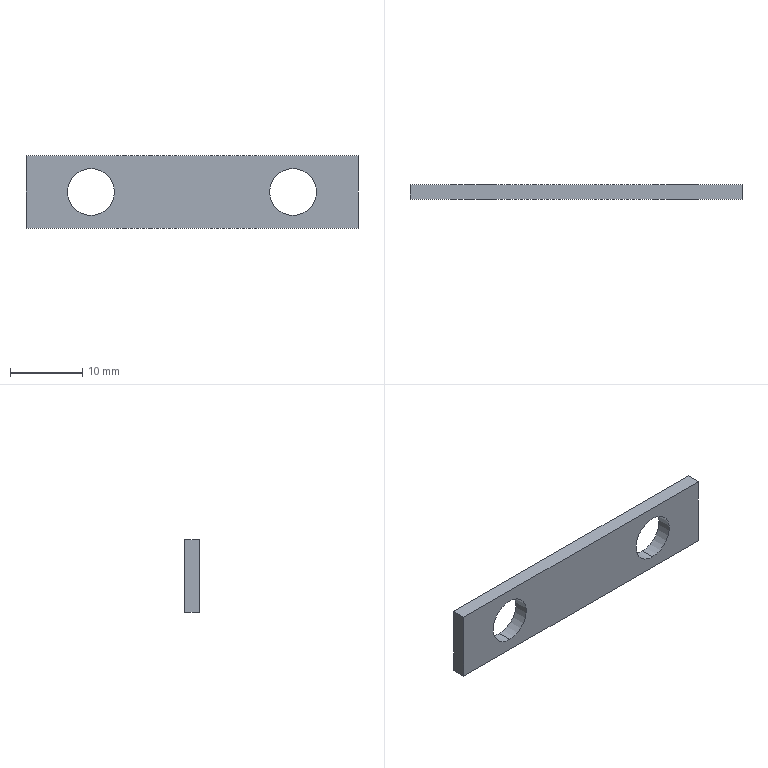Part | SolidWorks | features BaseBody 1 | 1 solid | 10 faces | box 46 x 2 x 10 mm | volume 787.268 mm3 | plane 6 | cylinder 4 | commonest cylinder face diameters 6.5 x4
STEP:
#1=CARTESIAN_POINT('',(14.,2.,3.25));
#2=VERTEX_POINT('',#1);
#3=CARTESIAN_POINT('',(14.,2.,-3.25));
#4=VERTEX_POINT('',#3);
#5=CARTESIAN_POINT('',(14.,2.,0.));
#6=DIRECTION('',(0.,-1.,0.));
#7=DIRECTION('',(0.,0.,1.));
#8=AXIS2_PLACEMENT_3D('',#5,#6,#7);
#9=CIRCLE('',#8,3.25);
#10=EDGE_CURVE('',#2,#4,#9,.T.);
#11=ORIENTED_EDGE('',*,*,#10,.T.);
#12=CARTESIAN_POINT('',(14.,2.,0.));
#13=DIRECTION('',(0.,-1.,0.));
#14=DIRECTION('',(0.,0.,1.));
#15=AXIS2_PLACEMENT_3D('',#12,#13,#14);
#16=CIRCLE('',#15,3.25);
#17=EDGE_CURVE('',#4,#2,#16,.T.);
#18=ORIENTED_EDGE('',*,*,#17,.T.);
#19=EDGE_LOOP('',(#11,#18));
#20=FACE_BOUND('',#19,.T.);
#21=CARTESIAN_POINT('',(-14.,2.,3.25));
#22=VERTEX_POINT('',#21);
#23=CARTESIAN_POINT('',(-14.,2.,-3.25));
#24=VERTEX_POINT('',#23);
#25=CARTESIAN_POINT('',(-14.,2.,0.));
#26=DIRECTION('',(0.,-1.,0.));
#27=DIRECTION('',(0.,0.,1.));
#28=AXIS2_PLACEMENT_3D('',#25,#26,#27);
#29=CIRCLE('',#28,3.25);
#30=EDGE_CURVE('',#22,#24,#29,.T.);
#31=ORIENTED_EDGE('',*,*,#30,.T.);
#32=CARTESIAN_POINT('',(-14.,2.,0.));
#33=DIRECTION('',(0.,-1.,0.));
#34=DIRECTION('',(0.,0.,1.));
#35=AXIS2_PLACEMENT_3D('',#32,#33,#34);
#36=CIRCLE('',#35,3.25);
#37=EDGE_CURVE('',#24,#22,#36,.T.);
#38=ORIENTED_EDGE('',*,*,#37,.T.);
#39=EDGE_LOOP('',(#31,#38));
#40=FACE_BOUND('',#39,.T.);
#41=CARTESIAN_POINT('',(23.,2.,5.));
#42=VERTEX_POINT('',#41);
#43=CARTESIAN_POINT('',(23.,2.,-5.));
#44=VERTEX_POINT('',#43);
#45=CARTESIAN_POINT('',(23.,2.,-5.));
#46=DIRECTION('',(0.,0.,-1.));
#47=VECTOR('',#46,1000.);
#48=LINE('',#45,#47);
#49=EDGE_CURVE('',#42,#44,#48,.T.);
#50=ORIENTED_EDGE('',*,*,#49,.T.);
#51=CARTESIAN_POINT('',(-23.,2.,-5.));
#52=VERTEX_POINT('',#51);
#53=CARTESIAN_POINT('',(-23.,2.,-5.));
#54=DIRECTION('',(-1.,0.,0.));
#55=VECTOR('',#54,1000.);
#56=LINE('',#53,#55);
#57=EDGE_CURVE('',#44,#52,#56,.T.);
#58=ORIENTED_EDGE('',*,*,#57,.T.);
#59=CARTESIAN_POINT('',(-23.,2.,5.));
#60=VERTEX_POINT('',#59);
#61=CARTESIAN_POINT('',(-23.,2.,-5.));
#62=DIRECTION('',(0.,0.,1.));
#63=VECTOR('',#62,1000.);
#64=LINE('',#61,#63);
#65=EDGE_CURVE('',#52,#60,#64,.T.);
#66=ORIENTED_EDGE('',*,*,#65,.T.);
#67=CARTESIAN_POINT('',(-23.,2.,5.));
#68=DIRECTION('',(1.,0.,0.));
#69=VECTOR('',#68,1000.);
#70=LINE('',#67,#69);
#71=EDGE_CURVE('',#60,#42,#70,.T.);
#72=ORIENTED_EDGE('',*,*,#71,.T.);
#73=EDGE_LOOP('',(#50,#58,#66,#72));
#74=FACE_OUTER_BOUND('',#73,.T.);
#75=CARTESIAN_POINT('',(0.,2.,0.));
#76=DIRECTION('',(0.,1.,0.));
#77=DIRECTION('',(1.,0.,0.));
#78=AXIS2_PLACEMENT_3D('',#75,#76,#77);
#79=PLANE('',#78);
#80=ADVANCED_FACE('',(#20,#40,#74),#79,.T.);
#81=ORIENTED_EDGE('',*,*,#49,.F.);
#82=CARTESIAN_POINT('',(23.,0.,5.));
#83=VERTEX_POINT('',#82);
#84=CARTESIAN_POINT('',(23.,2.,5.));
#85=DIRECTION('',(0.,-1.,0.));
#86=VECTOR('',#85,1000.);
#87=LINE('',#84,#86);
#88=EDGE_CURVE('',#42,#83,#87,.T.);
#89=ORIENTED_EDGE('',*,*,#88,.T.);
#90=CARTESIAN_POINT('',(23.,0.,-5.));
#91=VERTEX_POINT('',#90);
#92=CARTESIAN_POINT('',(23.,0.,0.));
#93=DIRECTION('',(0.,0.,-1.));
#94=VECTOR('',#93,1000.);
#95=LINE('',#92,#94);
#96=EDGE_CURVE('',#83,#91,#95,.T.);
#97=ORIENTED_EDGE('',*,*,#96,.T.);
#98=CARTESIAN_POINT('',(23.,2.,-5.));
#99=DIRECTION('',(0.,1.,0.));
#100=VECTOR('',#99,1000.);
#101=LINE('',#98,#100);
#102=EDGE_CURVE('',#91,#44,#101,.T.);
#103=ORIENTED_EDGE('',*,*,#102,.T.);
#104=EDGE_LOOP('',(#81,#89,#97,#103));
#105=FACE_OUTER_BOUND('',#104,.T.);
#106=CARTESIAN_POINT('',(23.,2.,-5.));
#107=DIRECTION('',(-1.,0.,0.));
#108=DIRECTION('',(0.,0.,1.));
#109=AXIS2_PLACEMENT_3D('',#106,#107,#108);
#110=PLANE('',#109);
#111=ADVANCED_FACE('',(#105),#110,.F.);
#112=ORIENTED_EDGE('',*,*,#57,.F.);
#113=ORIENTED_EDGE('',*,*,#102,.F.);
#114=CARTESIAN_POINT('',(-23.,0.,-5.));
#115=VERTEX_POINT('',#114);
#116=CARTESIAN_POINT('',(0.,0.,-5.));
#117=DIRECTION('',(-1.,0.,0.));
#118=VECTOR('',#117,1000.);
#119=LINE('',#116,#118);
#120=EDGE_CURVE('',#91,#115,#119,.T.);
#121=ORIENTED_EDGE('',*,*,#120,.T.);
#122=CARTESIAN_POINT('',(-23.,2.,-5.));
#123=DIRECTION('',(0.,1.,0.));
#124=VECTOR('',#123,1000.);
#125=LINE('',#122,#124);
#126=EDGE_CURVE('',#115,#52,#125,.T.);
#127=ORIENTED_EDGE('',*,*,#126,.T.);
#128=EDGE_LOOP('',(#112,#113,#121,#127));
#129=FACE_OUTER_BOUND('',#128,.T.);
#130=CARTESIAN_POINT('',(-23.,2.,-5.));
#131=DIRECTION('',(0.,0.,1.));
#132=DIRECTION('',(1.,0.,0.));
#133=AXIS2_PLACEMENT_3D('',#130,#131,#132);
#134=PLANE('',#133);
#135=ADVANCED_FACE('',(#129),#134,.F.);
#136=ORIENTED_EDGE('',*,*,#65,.F.);
#137=ORIENTED_EDGE('',*,*,#126,.F.);
#138=CARTESIAN_POINT('',(-23.,0.,5.));
#139=VERTEX_POINT('',#138);
#140=CARTESIAN_POINT('',(-23.,0.,0.));
#141=DIRECTION('',(0.,0.,1.));
#142=VECTOR('',#141,1000.);
#143=LINE('',#140,#142);
#144=EDGE_CURVE('',#115,#139,#143,.T.);
#145=ORIENTED_EDGE('',*,*,#144,.T.);
#146=CARTESIAN_POINT('',(-23.,2.,5.));
#147=DIRECTION('',(0.,1.,0.));
#148=VECTOR('',#147,1000.);
#149=LINE('',#146,#148);
#150=EDGE_CURVE('',#139,#60,#149,.T.);
#151=ORIENTED_EDGE('',*,*,#150,.T.);
#152=EDGE_LOOP('',(#136,#137,#145,#151));
#153=FACE_OUTER_BOUND('',#152,.T.);
#154=CARTESIAN_POINT('',(-23.,2.,-5.));
#155=DIRECTION('',(1.,0.,0.));
#156=DIRECTION('',(0.,1.,0.));
#157=AXIS2_PLACEMENT_3D('',#154,#155,#156);
#158=PLANE('',#157);
#159=ADVANCED_FACE('',(#153),#158,.F.);
#160=ORIENTED_EDGE('',*,*,#71,.F.);
#161=ORIENTED_EDGE('',*,*,#150,.F.);
#162=CARTESIAN_POINT('',(0.,0.,5.));
#163=DIRECTION('',(1.,0.,0.));
#164=VECTOR('',#163,1000.);
#165=LINE('',#162,#164);
#166=EDGE_CURVE('',#139,#83,#165,.T.);
#167=ORIENTED_EDGE('',*,*,#166,.T.);
#168=ORIENTED_EDGE('',*,*,#88,.F.);
#169=EDGE_LOOP('',(#160,#161,#167,#168));
#170=FACE_OUTER_BOUND('',#169,.T.);
#171=CARTESIAN_POINT('',(-23.,2.,5.));
#172=DIRECTION('',(0.,0.,-1.));
#173=DIRECTION('',(0.,-1.,0.));
#174=AXIS2_PLACEMENT_3D('',#171,#172,#173);
#175=PLANE('',#174);
#176=ADVANCED_FACE('',(#170),#175,.F.);
#177=CARTESIAN_POINT('',(14.,0.,-3.25));
#178=VERTEX_POINT('',#177);
#179=CARTESIAN_POINT('',(14.,2.,-3.25));
#180=DIRECTION('',(0.,1.,0.));
#181=VECTOR('',#180,1000.);
#182=LINE('',#179,#181);
#183=EDGE_CURVE('',#178,#4,#182,.T.);
#184=ORIENTED_EDGE('',*,*,#183,.F.);
#185=CARTESIAN_POINT('',(14.,0.,3.25));
#186=VERTEX_POINT('',#185);
#187=CARTESIAN_POINT('',(14.,0.,0.));
#188=DIRECTION('',(0.,-1.,0.));
#189=DIRECTION('',(0.,0.,1.));
#190=AXIS2_PLACEMENT_3D('',#187,#188,#189);
#191=CIRCLE('',#190,3.25);
#192=EDGE_CURVE('',#178,#186,#191,.T.);
#193=ORIENTED_EDGE('',*,*,#192,.T.);
#194=CARTESIAN_POINT('',(14.,2.,3.25));
#195=DIRECTION('',(0.,1.,0.));
#196=VECTOR('',#195,1000.);
#197=LINE('',#194,#196);
#198=EDGE_CURVE('',#186,#2,#197,.T.);
#199=ORIENTED_EDGE('',*,*,#198,.T.);
#200=ORIENTED_EDGE('',*,*,#17,.F.);
#201=EDGE_LOOP('',(#184,#193,#199,#200));
#202=FACE_OUTER_BOUND('',#201,.T.);
#203=CARTESIAN_POINT('',(14.,2.,0.));
#204=DIRECTION('',(0.,1.,0.));
#205=DIRECTION('',(0.,0.,1.));
#206=AXIS2_PLACEMENT_3D('',#203,#204,#205);
#207=CYLINDRICAL_SURFACE('',#206,3.25);
#208=ADVANCED_FACE('',(#202),#207,.F.);
#209=CARTESIAN_POINT('',(-14.,0.,-3.25));
#210=VERTEX_POINT('',#209);
#211=CARTESIAN_POINT('',(-14.,2.,-3.25));
#212=DIRECTION('',(0.,1.,0.));
#213=VECTOR('',#212,1000.);
#214=LINE('',#211,#213);
#215=EDGE_CURVE('',#210,#24,#214,.T.);
#216=ORIENTED_EDGE('',*,*,#215,.F.);
#217=CARTESIAN_POINT('',(-14.,0.,3.25));
#218=VERTEX_POINT('',#217);
#219=CARTESIAN_POINT('',(-14.,0.,0.));
#220=DIRECTION('',(0.,-1.,0.));
#221=DIRECTION('',(0.,0.,1.));
#222=AXIS2_PLACEMENT_3D('',#219,#220,#221);
#223=CIRCLE('',#222,3.25);
#224=EDGE_CURVE('',#210,#218,#223,.T.);
#225=ORIENTED_EDGE('',*,*,#224,.T.);
#226=CARTESIAN_POINT('',(-14.,2.,3.25));
#227=DIRECTION('',(0.,1.,0.));
#228=VECTOR('',#227,1000.);
#229=LINE('',#226,#228);
#230=EDGE_CURVE('',#218,#22,#229,.T.);
#231=ORIENTED_EDGE('',*,*,#230,.T.);
#232=ORIENTED_EDGE('',*,*,#37,.F.);
#233=EDGE_LOOP('',(#216,#225,#231,#232));
#234=FACE_OUTER_BOUND('',#233,.T.);
#235=CARTESIAN_POINT('',(-14.,2.,0.));
#236=DIRECTION('',(0.,1.,0.));
#237=DIRECTION('',(0.,0.,1.));
#238=AXIS2_PLACEMENT_3D('',#235,#236,#237);
#239=CYLINDRICAL_SURFACE('',#238,3.25);
#240=ADVANCED_FACE('',(#234),#239,.F.);
#241=CARTESIAN_POINT('',(14.,0.,0.));
#242=DIRECTION('',(0.,-1.,0.));
#243=DIRECTION('',(0.,0.,1.));
#244=AXIS2_PLACEMENT_3D('',#241,#242,#243);
#245=CIRCLE('',#244,3.25);
#246=EDGE_CURVE('',#186,#178,#245,.T.);
#247=ORIENTED_EDGE('',*,*,#246,.F.);
#248=ORIENTED_EDGE('',*,*,#192,.F.);
#249=EDGE_LOOP('',(#247,#248));
#250=FACE_BOUND('',#249,.T.);
#251=CARTESIAN_POINT('',(-14.,0.,0.));
#252=DIRECTION('',(0.,-1.,0.));
#253=DIRECTION('',(0.,0.,1.));
#254=AXIS2_PLACEMENT_3D('',#251,#252,#253);
#255=CIRCLE('',#254,3.25);
#256=EDGE_CURVE('',#218,#210,#255,.T.);
#257=ORIENTED_EDGE('',*,*,#256,.F.);
#258=ORIENTED_EDGE('',*,*,#224,.F.);
#259=EDGE_LOOP('',(#257,#258));
#260=FACE_BOUND('',#259,.T.);
#261=ORIENTED_EDGE('',*,*,#144,.F.);
#262=ORIENTED_EDGE('',*,*,#120,.F.);
#263=ORIENTED_EDGE('',*,*,#96,.F.);
#264=ORIENTED_EDGE('',*,*,#166,.F.);
#265=EDGE_LOOP('',(#261,#262,#263,#264));
#266=FACE_OUTER_BOUND('',#265,.T.);
#267=CARTESIAN_POINT('',(0.,0.,0.));
#268=DIRECTION('',(0.,1.,0.));
#269=DIRECTION('',(1.,0.,0.));
#270=AXIS2_PLACEMENT_3D('',#267,#268,#269);
#271=PLANE('',#270);
#272=ADVANCED_FACE('',(#250,#260,#266),#271,.F.);
#273=ORIENTED_EDGE('',*,*,#246,.T.);
#274=ORIENTED_EDGE('',*,*,#183,.T.);
#275=ORIENTED_EDGE('',*,*,#10,.F.);
#276=ORIENTED_EDGE('',*,*,#198,.F.);
#277=EDGE_LOOP('',(#273,#274,#275,#276));
#278=FACE_OUTER_BOUND('',#277,.T.);
#279=CARTESIAN_POINT('',(14.,2.,0.));
#280=DIRECTION('',(0.,1.,0.));
#281=DIRECTION('',(0.,0.,1.));
#282=AXIS2_PLACEMENT_3D('',#279,#280,#281);
#283=CYLINDRICAL_SURFACE('',#282,3.25);
#284=ADVANCED_FACE('',(#278),#283,.F.);
#285=ORIENTED_EDGE('',*,*,#256,.T.);
#286=ORIENTED_EDGE('',*,*,#215,.T.);
#287=ORIENTED_EDGE('',*,*,#30,.F.);
#288=ORIENTED_EDGE('',*,*,#230,.F.);
#289=EDGE_LOOP('',(#285,#286,#287,#288));
#290=FACE_OUTER_BOUND('',#289,.T.);
#291=CARTESIAN_POINT('',(-14.,2.,0.));
#292=DIRECTION('',(0.,1.,0.));
#293=DIRECTION('',(0.,0.,1.));
#294=AXIS2_PLACEMENT_3D('',#291,#292,#293);
#295=CYLINDRICAL_SURFACE('',#294,3.25);
#296=ADVANCED_FACE('',(#290),#295,.F.);
#297=CLOSED_SHELL('',(#80,#111,#135,#159,#176,#208,#240,#272,#284,#296));
#298=MANIFOLD_SOLID_BREP('',#297);
#299=CARTESIAN_POINT('',(0.,0.,0.));
#300=DIRECTION('',(0.,0.,1.));
#301=DIRECTION('',(1.,0.,0.));
#302=AXIS2_PLACEMENT_3D('',#299,#300,#301);
#303=(LENGTH_UNIT()NAMED_UNIT(*)SI_UNIT(.MILLI.,.METRE.));
#304=UNCERTAINTY_MEASURE_WITH_UNIT(LENGTH_MEASURE(0.00001),#303,'','');
#305=(NAMED_UNIT(*)PLANE_ANGLE_UNIT()SI_UNIT($,.RADIAN.));
#306=(NAMED_UNIT(*)SI_UNIT($,.STERADIAN.)SOLID_ANGLE_UNIT());
#307=(GEOMETRIC_REPRESENTATION_CONTEXT(3)GLOBAL_UNCERTAINTY_ASSIGNED_CONTEXT((#304))GLOBAL_UNIT_ASSIGNED_CONTEXT((#303,#305,#306))REPRESENTATION_CONTEXT('',''));
#308=ADVANCED_BREP_SHAPE_REPRESENTATION('',(#298,#302),#307);